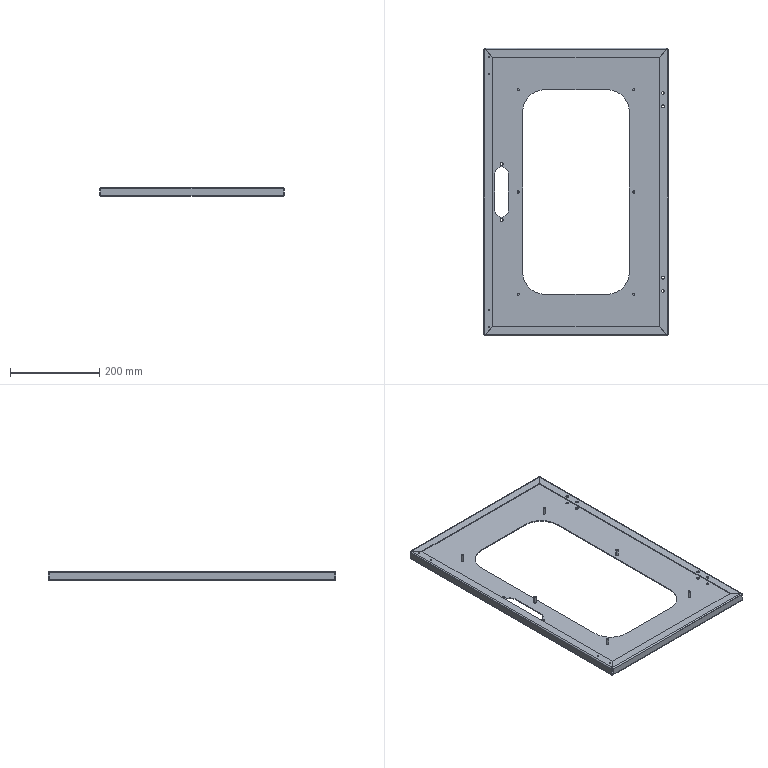Part | SolidWorks | features HoleWzd 3, ICE 3, EdgeFlange 2, Cut 1, FlatPattern 1, LPattern 1, SMBaseFlange 1, SheetMetal 1 | 1 solid | 128 faces | box 414.5 x 646 x 20 mm | volume 455877 mm3 | cylinder 62 | plane 50 | spline 16 | commonest cylinder face diameters 6.5 x16 5 x12 1.473 x8 3.3 x8 5.473 x8 7 x4